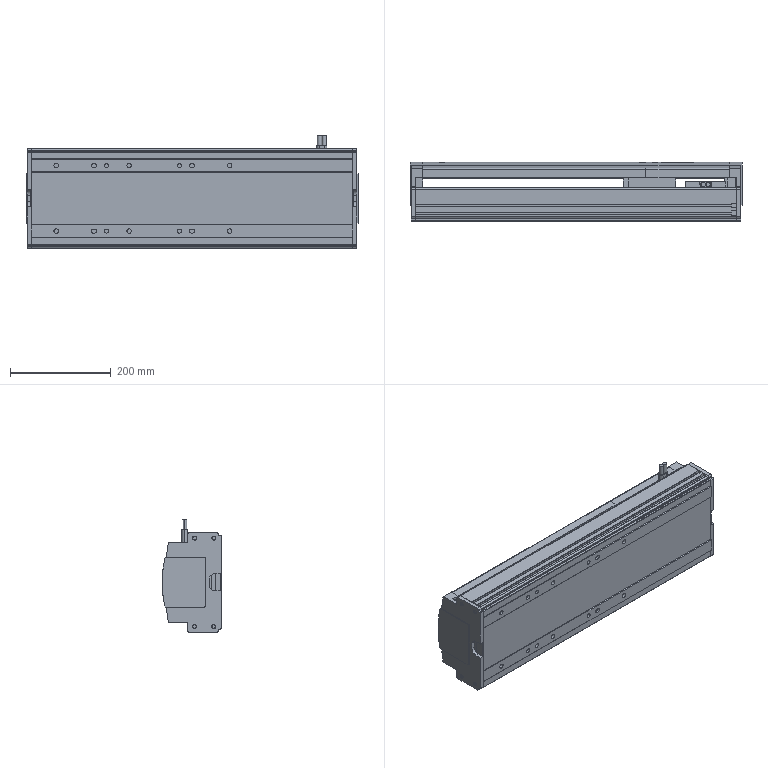Part | STEP file | ISPB-WXM-WA-750-10-200-T4-N-A1-AQ-B-EB^-Part-1 | 1 solid | 462 faces | box 660 x 118.5 x 223.4 mm | volume 8521972 mm3 | plane 295 | cylinder 167 | commonest cylinder face diameters 8 x32 9 x28 7 x16 7.6 x16 6 x12 18 x12